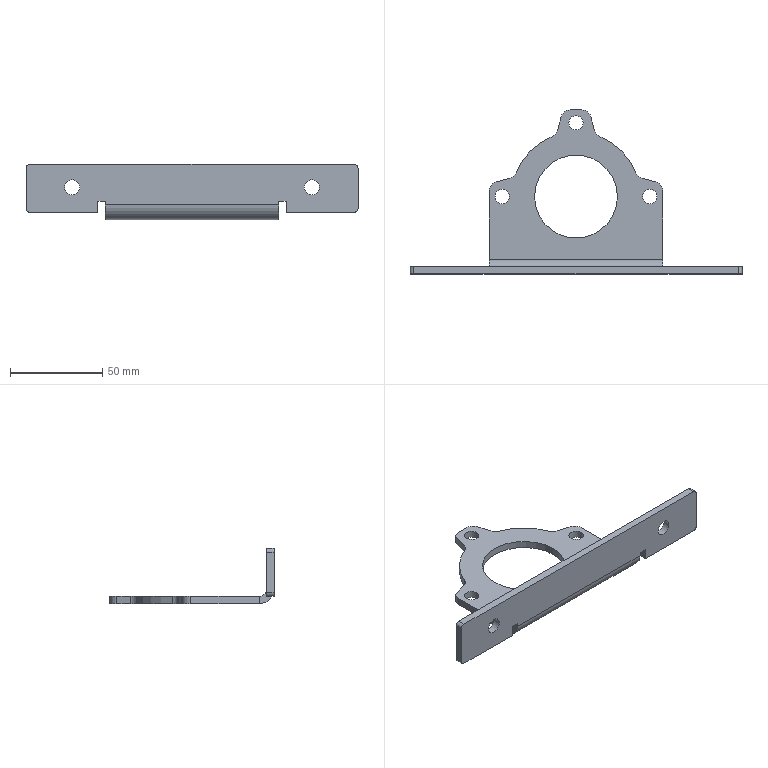Part | STEP file | Support gearmotor part1 B | 1 solid | 46 faces | box 180 x 89 x 30 mm | volume 35388 mm3 | plane 24 | cylinder 22 | commonest cylinder face diameters 10 x8 4 x4 7.8 x3 8.2 x2 70 x2 8 x1